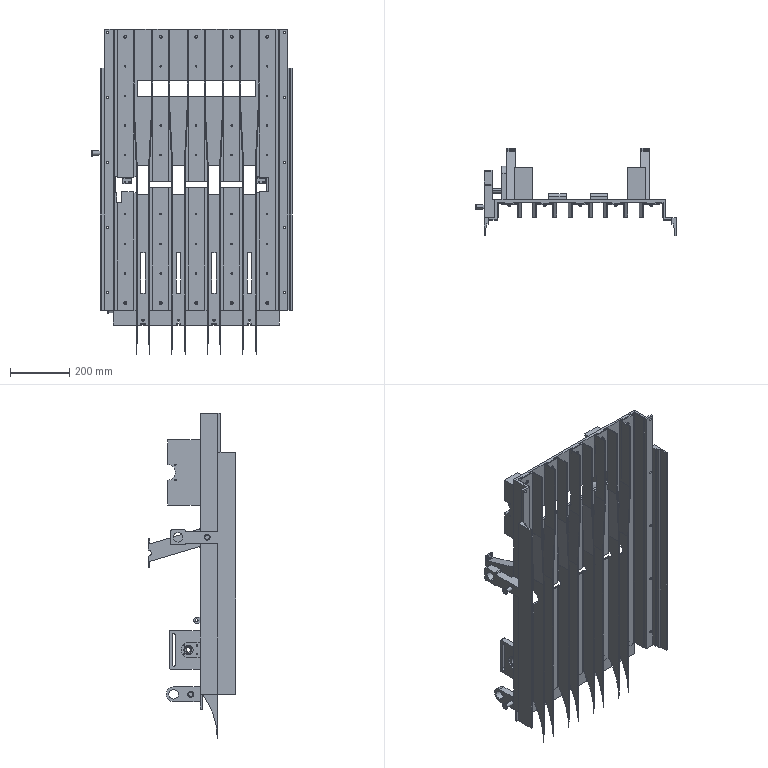Part | SolidWorks | 16 solids | 1353 faces | box 678.27 x 295.879 x 1100 mm | volume 12363792 mm3 | cylinder 625 | plane 560 | sphere 120 | torus 28 | cone 20 | commonest cylinder face diameters 0.5 x240 5 x208 8 x44 10 x44 3 x32 20 x12